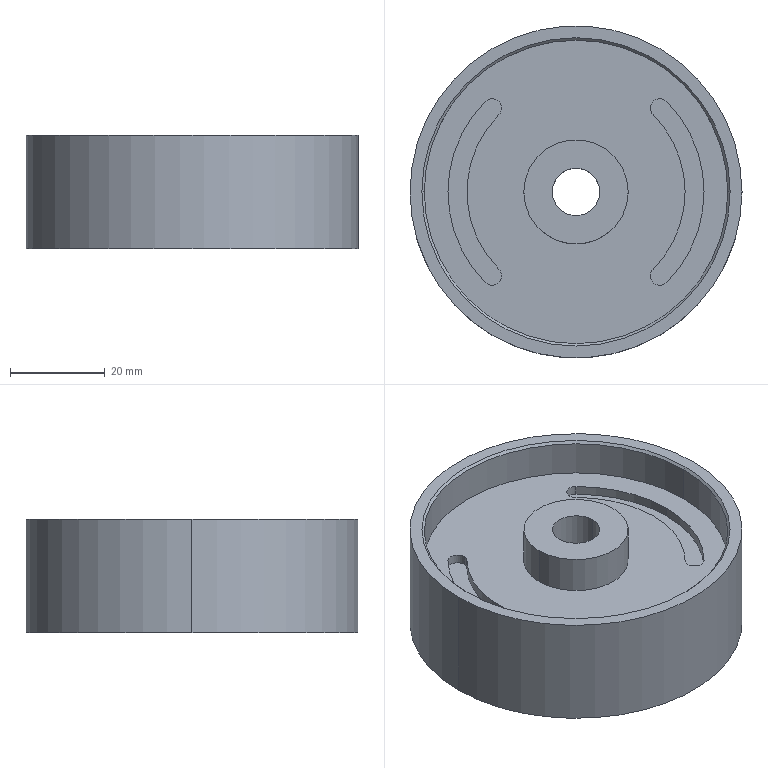Part | SolidWorks | features ICE 3, MirrorPattern 2, Chamfer 1, Extrusion 1 | 1 solid | 50 faces | box 70 x 70 x 24 mm | volume 43680 mm3 | cylinder 36 | plane 10 | cone 4 | commonest cylinder face diameters 4 x12 46 x6 54 x6 22 x4 64 x4 10 x2
STEP:
#1=CARTESIAN_POINT('',(-32.,0.,11.5));
#2=VERTEX_POINT('',#1);
#3=CARTESIAN_POINT('',(32.,0.,11.5));
#4=VERTEX_POINT('',#3);
#5=CARTESIAN_POINT('',(0.,0.,11.5));
#6=DIRECTION('',(0.,0.,1.));
#7=DIRECTION('',(1.,0.,0.));
#8=AXIS2_PLACEMENT_3D('',#5,#6,#7);
#9=CIRCLE('',#8,32.);
#10=EDGE_CURVE('',#2,#4,#9,.T.);
#11=ORIENTED_EDGE('',*,*,#10,.F.);
#12=CARTESIAN_POINT('',(-32.5,0.,12.));
#13=VERTEX_POINT('',#12);
#14=CARTESIAN_POINT('',(-32.,0.,11.5));
#15=DIRECTION('',(-0.7071,0.,0.7071));
#16=VECTOR('',#15,1000.);
#17=LINE('',#14,#16);
#18=EDGE_CURVE('',#2,#13,#17,.T.);
#19=ORIENTED_EDGE('',*,*,#18,.T.);
#20=CARTESIAN_POINT('',(32.5,0.,12.));
#21=VERTEX_POINT('',#20);
#22=CARTESIAN_POINT('',(0.,0.,12.));
#23=DIRECTION('',(0.,0.,-1.));
#24=DIRECTION('',(1.,0.,0.));
#25=AXIS2_PLACEMENT_3D('',#22,#23,#24);
#26=CIRCLE('',#25,32.5);
#27=EDGE_CURVE('',#21,#13,#26,.T.);
#28=ORIENTED_EDGE('',*,*,#27,.F.);
#29=CARTESIAN_POINT('',(32.,0.,11.5));
#30=DIRECTION('',(0.7071,0.,0.7071));
#31=VECTOR('',#30,1000.);
#32=LINE('',#29,#31);
#33=EDGE_CURVE('',#4,#21,#32,.T.);
#34=ORIENTED_EDGE('',*,*,#33,.F.);
#35=EDGE_LOOP('',(#11,#19,#28,#34));
#36=FACE_OUTER_BOUND('',#35,.T.);
#37=CARTESIAN_POINT('',(0.,0.,11.5));
#38=DIRECTION('',(0.,0.,1.));
#39=DIRECTION('',(1.,0.,0.));
#40=AXIS2_PLACEMENT_3D('',#37,#38,#39);
#41=CONICAL_SURFACE('',#40,32.,0.7854);
#42=ADVANCED_FACE('',(#36),#41,.F.);
#43=CARTESIAN_POINT('',(32.,0.,-11.5));
#44=VERTEX_POINT('',#43);
#45=CARTESIAN_POINT('',(-32.,0.,-11.5));
#46=VERTEX_POINT('',#45);
#47=CARTESIAN_POINT('',(0.,0.,-11.5));
#48=DIRECTION('',(0.,0.,-1.));
#49=DIRECTION('',(1.,0.,0.));
#50=AXIS2_PLACEMENT_3D('',#47,#48,#49);
#51=CIRCLE('',#50,32.);
#52=EDGE_CURVE('',#44,#46,#51,.T.);
#53=ORIENTED_EDGE('',*,*,#52,.F.);
#54=CARTESIAN_POINT('',(32.5,0.,-12.));
#55=VERTEX_POINT('',#54);
#56=CARTESIAN_POINT('',(32.5,0.,-12.));
#57=DIRECTION('',(0.7071,0.,-0.7071));
#58=VECTOR('',#57,1000.);
#59=LINE('',#56,#58);
#60=EDGE_CURVE('',#44,#55,#59,.T.);
#61=ORIENTED_EDGE('',*,*,#60,.T.);
#62=CARTESIAN_POINT('',(-32.5,0.,-12.));
#63=VERTEX_POINT('',#62);
#64=CARTESIAN_POINT('',(0.,0.,-12.));
#65=DIRECTION('',(0.,0.,1.));
#66=DIRECTION('',(1.,0.,0.));
#67=AXIS2_PLACEMENT_3D('',#64,#65,#66);
#68=CIRCLE('',#67,32.5);
#69=EDGE_CURVE('',#63,#55,#68,.T.);
#70=ORIENTED_EDGE('',*,*,#69,.F.);
#71=CARTESIAN_POINT('',(-32.5,0.,-12.));
#72=DIRECTION('',(-0.7071,0.,-0.7071));
#73=VECTOR('',#72,1000.);
#74=LINE('',#71,#73);
#75=EDGE_CURVE('',#46,#63,#74,.T.);
#76=ORIENTED_EDGE('',*,*,#75,.F.);
#77=EDGE_LOOP('',(#53,#61,#70,#76));
#78=FACE_OUTER_BOUND('',#77,.T.);
#79=CARTESIAN_POINT('',(0.,0.,-12.));
#80=DIRECTION('',(0.,0.,-1.));
#81=DIRECTION('',(-1.,0.,0.));
#82=AXIS2_PLACEMENT_3D('',#79,#80,#81);
#83=CONICAL_SURFACE('',#82,32.5,0.7854);
#84=ADVANCED_FACE('',(#78),#83,.F.);
#85=CARTESIAN_POINT('',(-19.092,19.092,2.));
#86=VERTEX_POINT('',#85);
#87=CARTESIAN_POINT('',(-15.678,17.678,2.));
#88=VERTEX_POINT('',#87);
#89=CARTESIAN_POINT('',(-17.678,17.678,2.));
#90=DIRECTION('',(0.,0.,-1.));
#91=DIRECTION('',(-1.,0.,0.));
#92=AXIS2_PLACEMENT_3D('',#89,#90,#91);
#93=CIRCLE('',#92,2.);
#94=EDGE_CURVE('',#86,#88,#93,.T.);
#95=ORIENTED_EDGE('',*,*,#94,.T.);
#96=CARTESIAN_POINT('',(-15.678,17.678,4.));
#97=VERTEX_POINT('',#96);
#98=CARTESIAN_POINT('',(-15.678,17.678,2.));
#99=DIRECTION('',(0.,0.,1.));
#100=VECTOR('',#99,1000.);
#101=LINE('',#98,#100);
#102=EDGE_CURVE('',#88,#97,#101,.T.);
#103=ORIENTED_EDGE('',*,*,#102,.T.);
#104=CARTESIAN_POINT('',(-19.092,19.092,4.));
#105=VERTEX_POINT('',#104);
#106=CARTESIAN_POINT('',(-17.678,17.678,4.));
#107=DIRECTION('',(0.,0.,-1.));
#108=DIRECTION('',(-1.,0.,0.));
#109=AXIS2_PLACEMENT_3D('',#106,#107,#108);
#110=CIRCLE('',#109,2.);
#111=EDGE_CURVE('',#105,#97,#110,.T.);
#112=ORIENTED_EDGE('',*,*,#111,.F.);
#113=CARTESIAN_POINT('',(-19.092,19.092,2.));
#114=DIRECTION('',(0.,0.,1.));
#115=VECTOR('',#114,1000.);
#116=LINE('',#113,#115);
#117=EDGE_CURVE('',#86,#105,#116,.T.);
#118=ORIENTED_EDGE('',*,*,#117,.F.);
#119=EDGE_LOOP('',(#95,#103,#112,#118));
#120=FACE_OUTER_BOUND('',#119,.T.);
#121=CARTESIAN_POINT('',(-17.678,17.678,2.));
#122=DIRECTION('',(0.,0.,1.));
#123=DIRECTION('',(1.,0.,0.));
#124=AXIS2_PLACEMENT_3D('',#121,#122,#123);
#125=CYLINDRICAL_SURFACE('',#124,2.);
#126=ADVANCED_FACE('',(#120),#125,.F.);
#127=CARTESIAN_POINT('',(-16.263,-16.263,2.));
#128=VERTEX_POINT('',#127);
#129=CARTESIAN_POINT('',(-15.678,-17.678,2.));
#130=VERTEX_POINT('',#129);
#131=CARTESIAN_POINT('',(-17.678,-17.678,2.));
#132=DIRECTION('',(0.,0.,-1.));
#133=DIRECTION('',(-1.,0.,0.));
#134=AXIS2_PLACEMENT_3D('',#131,#132,#133);
#135=CIRCLE('',#134,2.);
#136=EDGE_CURVE('',#128,#130,#135,.T.);
#137=ORIENTED_EDGE('',*,*,#136,.T.);
#138=CARTESIAN_POINT('',(-15.678,-17.678,4.));
#139=VERTEX_POINT('',#138);
#140=CARTESIAN_POINT('',(-15.678,-17.678,2.));
#141=DIRECTION('',(0.,0.,1.));
#142=VECTOR('',#141,1000.);
#143=LINE('',#140,#142);
#144=EDGE_CURVE('',#130,#139,#143,.T.);
#145=ORIENTED_EDGE('',*,*,#144,.T.);
#146=CARTESIAN_POINT('',(-16.263,-16.263,4.));
#147=VERTEX_POINT('',#146);
#148=CARTESIAN_POINT('',(-17.678,-17.678,4.));
#149=DIRECTION('',(0.,0.,-1.));
#150=DIRECTION('',(-1.,0.,0.));
#151=AXIS2_PLACEMENT_3D('',#148,#149,#150);
#152=CIRCLE('',#151,2.);
#153=EDGE_CURVE('',#147,#139,#152,.T.);
#154=ORIENTED_EDGE('',*,*,#153,.F.);
#155=CARTESIAN_POINT('',(-16.263,-16.263,2.));
#156=DIRECTION('',(0.,0.,1.));
#157=VECTOR('',#156,1000.);
#158=LINE('',#155,#157);
#159=EDGE_CURVE('',#128,#147,#158,.T.);
#160=ORIENTED_EDGE('',*,*,#159,.F.);
#161=EDGE_LOOP('',(#137,#145,#154,#160));
#162=FACE_OUTER_BOUND('',#161,.T.);
#163=CARTESIAN_POINT('',(-17.678,-17.678,2.));
#164=DIRECTION('',(0.,0.,1.));
#165=DIRECTION('',(1.,0.,0.));
#166=AXIS2_PLACEMENT_3D('',#163,#164,#165);
#167=CYLINDRICAL_SURFACE('',#166,2.);
#168=ADVANCED_FACE('',(#162),#167,.F.);
#169=CARTESIAN_POINT('',(19.092,19.092,2.));
#170=VERTEX_POINT('',#169);
#171=CARTESIAN_POINT('',(27.,0.,2.));
#172=VERTEX_POINT('',#171);
#173=CARTESIAN_POINT('',(0.,0.,2.));
#174=DIRECTION('',(0.,0.,-1.));
#175=DIRECTION('',(1.,0.,0.));
#176=AXIS2_PLACEMENT_3D('',#173,#174,#175);
#177=CIRCLE('',#176,27.);
#178=EDGE_CURVE('',#170,#172,#177,.T.);
#179=ORIENTED_EDGE('',*,*,#178,.T.);
#180=CARTESIAN_POINT('',(27.,0.,4.));
#181=VERTEX_POINT('',#180);
#182=CARTESIAN_POINT('',(27.,0.,2.));
#183=DIRECTION('',(0.,0.,1.));
#184=VECTOR('',#183,1000.);
#185=LINE('',#182,#184);
#186=EDGE_CURVE('',#172,#181,#185,.T.);
#187=ORIENTED_EDGE('',*,*,#186,.T.);
#188=CARTESIAN_POINT('',(19.092,19.092,4.));
#189=VERTEX_POINT('',#188);
#190=CARTESIAN_POINT('',(0.,0.,4.));
#191=DIRECTION('',(0.,0.,-1.));
#192=DIRECTION('',(1.,0.,0.));
#193=AXIS2_PLACEMENT_3D('',#190,#191,#192);
#194=CIRCLE('',#193,27.);
#195=EDGE_CURVE('',#189,#181,#194,.T.);
#196=ORIENTED_EDGE('',*,*,#195,.F.);
#197=CARTESIAN_POINT('',(19.092,19.092,2.));
#198=DIRECTION('',(0.,0.,1.));
#199=VECTOR('',#198,1000.);
#200=LINE('',#197,#199);
#201=EDGE_CURVE('',#170,#189,#200,.T.);
#202=ORIENTED_EDGE('',*,*,#201,.F.);
#203=EDGE_LOOP('',(#179,#187,#196,#202));
#204=FACE_OUTER_BOUND('',#203,.T.);
#205=CARTESIAN_POINT('',(0.,0.,2.));
#206=DIRECTION('',(0.,0.,1.));
#207=DIRECTION('',(1.,0.,0.));
#208=AXIS2_PLACEMENT_3D('',#205,#206,#207);
#209=CYLINDRICAL_SURFACE('',#208,27.);
#210=ADVANCED_FACE('',(#204),#209,.F.);
#211=CARTESIAN_POINT('',(16.263,-16.263,2.));
#212=VERTEX_POINT('',#211);
#213=CARTESIAN_POINT('',(23.,0.,2.));
#214=VERTEX_POINT('',#213);
#215=CARTESIAN_POINT('',(0.,0.,2.));
#216=DIRECTION('',(0.,0.,1.));
#217=DIRECTION('',(1.,0.,0.));
#218=AXIS2_PLACEMENT_3D('',#215,#216,#217);
#219=CIRCLE('',#218,23.);
#220=EDGE_CURVE('',#212,#214,#219,.T.);
#221=ORIENTED_EDGE('',*,*,#220,.T.);
#222=CARTESIAN_POINT('',(23.,0.,4.));
#223=VERTEX_POINT('',#222);
#224=CARTESIAN_POINT('',(23.,0.,2.));
#225=DIRECTION('',(0.,0.,1.));
#226=VECTOR('',#225,1000.);
#227=LINE('',#224,#226);
#228=EDGE_CURVE('',#214,#223,#227,.T.);
#229=ORIENTED_EDGE('',*,*,#228,.T.);
#230=CARTESIAN_POINT('',(16.263,-16.263,4.));
#231=VERTEX_POINT('',#230);
#232=CARTESIAN_POINT('',(0.,0.,4.));
#233=DIRECTION('',(0.,0.,1.));
#234=DIRECTION('',(1.,0.,0.));
#235=AXIS2_PLACEMENT_3D('',#232,#233,#234);
#236=CIRCLE('',#235,23.);
#237=EDGE_CURVE('',#231,#223,#236,.T.);
#238=ORIENTED_EDGE('',*,*,#237,.F.);
#239=CARTESIAN_POINT('',(16.263,-16.263,2.));
#240=DIRECTION('',(0.,0.,1.));
#241=VECTOR('',#240,1000.);
#242=LINE('',#239,#241);
#243=EDGE_CURVE('',#212,#231,#242,.T.);
#244=ORIENTED_EDGE('',*,*,#243,.F.);
#245=EDGE_LOOP('',(#221,#229,#238,#244));
#246=FACE_OUTER_BOUND('',#245,.T.);
#247=CARTESIAN_POINT('',(0.,0.,2.));
#248=DIRECTION('',(0.,0.,1.));
#249=DIRECTION('',(1.,0.,0.));
#250=AXIS2_PLACEMENT_3D('',#247,#248,#249);
#251=CYLINDRICAL_SURFACE('',#250,23.);
#252=ADVANCED_FACE('',(#246),#251,.T.);
#253=CARTESIAN_POINT('',(-27.,0.,-2.));
#254=VERTEX_POINT('',#253);
#255=CARTESIAN_POINT('',(-19.092,19.092,-2.));
#256=VERTEX_POINT('',#255);
#257=CARTESIAN_POINT('',(0.,0.,-2.));
#258=DIRECTION('',(0.,0.,-1.));
#259=DIRECTION('',(-1.,0.,0.));
#260=AXIS2_PLACEMENT_3D('',#257,#258,#259);
#261=CIRCLE('',#260,27.);
#262=EDGE_CURVE('',#254,#256,#261,.T.);
#263=ORIENTED_EDGE('',*,*,#262,.F.);
#264=CARTESIAN_POINT('',(-27.,0.,-4.));
#265=VERTEX_POINT('',#264);
#266=CARTESIAN_POINT('',(-27.,0.,-2.));
#267=DIRECTION('',(0.,0.,-1.));
#268=VECTOR('',#267,1000.);
#269=LINE('',#266,#268);
#270=EDGE_CURVE('',#254,#265,#269,.T.);
#271=ORIENTED_EDGE('',*,*,#270,.T.);
#272=CARTESIAN_POINT('',(-19.092,19.092,-4.));
#273=VERTEX_POINT('',#272);
#274=CARTESIAN_POINT('',(0.,0.,-4.));
#275=DIRECTION('',(0.,0.,-1.));
#276=DIRECTION('',(-1.,0.,0.));
#277=AXIS2_PLACEMENT_3D('',#274,#275,#276);
#278=CIRCLE('',#277,27.);
#279=EDGE_CURVE('',#265,#273,#278,.T.);
#280=ORIENTED_EDGE('',*,*,#279,.T.);
#281=CARTESIAN_POINT('',(-19.092,19.092,-2.));
#282=DIRECTION('',(0.,0.,-1.));
#283=VECTOR('',#282,1000.);
#284=LINE('',#281,#283);
#285=EDGE_CURVE('',#256,#273,#284,.T.);
#286=ORIENTED_EDGE('',*,*,#285,.F.);
#287=EDGE_LOOP('',(#263,#271,#280,#286));
#288=FACE_OUTER_BOUND('',#287,.T.);
#289=CARTESIAN_POINT('',(0.,0.,-2.));
#290=DIRECTION('',(0.,0.,-1.));
#291=DIRECTION('',(-1.,0.,0.));
#292=AXIS2_PLACEMENT_3D('',#289,#290,#291);
#293=CYLINDRICAL_SURFACE('',#292,27.);
#294=ADVANCED_FACE('',(#288),#293,.F.);
#295=CARTESIAN_POINT('',(-23.,0.,-2.));
#296=VERTEX_POINT('',#295);
#297=CARTESIAN_POINT('',(-16.263,-16.263,-2.));
#298=VERTEX_POINT('',#297);
#299=CARTESIAN_POINT('',(0.,0.,-2.));
#300=DIRECTION('',(0.,0.,1.));
#301=DIRECTION('',(-1.,0.,0.));
#302=AXIS2_PLACEMENT_3D('',#299,#300,#301);
#303=CIRCLE('',#302,23.);
#304=EDGE_CURVE('',#296,#298,#303,.T.);
#305=ORIENTED_EDGE('',*,*,#304,.F.);
#306=CARTESIAN_POINT('',(-23.,0.,-4.));
#307=VERTEX_POINT('',#306);
#308=CARTESIAN_POINT('',(-23.,0.,-2.));
#309=DIRECTION('',(0.,0.,-1.));
#310=VECTOR('',#309,1000.);
#311=LINE('',#308,#310);
#312=EDGE_CURVE('',#296,#307,#311,.T.);
#313=ORIENTED_EDGE('',*,*,#312,.T.);
#314=CARTESIAN_POINT('',(-16.263,-16.263,-4.));
#315=VERTEX_POINT('',#314);
#316=CARTESIAN_POINT('',(0.,0.,-4.));
#317=DIRECTION('',(0.,0.,1.));
#318=DIRECTION('',(-1.,0.,0.));
#319=AXIS2_PLACEMENT_3D('',#316,#317,#318);
#320=CIRCLE('',#319,23.);
#321=EDGE_CURVE('',#307,#315,#320,.T.);
#322=ORIENTED_EDGE('',*,*,#321,.T.);
#323=CARTESIAN_POINT('',(-16.263,-16.263,-2.));
#324=DIRECTION('',(0.,0.,-1.));
#325=VECTOR('',#324,1000.);
#326=LINE('',#323,#325);
#327=EDGE_CURVE('',#298,#315,#326,.T.);
#328=ORIENTED_EDGE('',*,*,#327,.F.);
#329=EDGE_LOOP('',(#305,#313,#322,#328));
#330=FACE_OUTER_BOUND('',#329,.T.);
#331=CARTESIAN_POINT('',(0.,0.,-2.));
#332=DIRECTION('',(0.,0.,-1.));
#333=DIRECTION('',(-1.,0.,0.));
#334=AXIS2_PLACEMENT_3D('',#331,#332,#333);
#335=CYLINDRICAL_SURFACE('',#334,23.);
#336=ADVANCED_FACE('',(#330),#335,.T.);
#337=CARTESIAN_POINT('',(15.678,17.678,-2.));
#338=VERTEX_POINT('',#337);
#339=CARTESIAN_POINT('',(19.092,19.092,-2.));
#340=VERTEX_POINT('',#339);
#341=CARTESIAN_POINT('',(17.678,17.678,-2.));
#342=DIRECTION('',(0.,0.,-1.));
#343=DIRECTION('',(1.,0.,0.));
#344=AXIS2_PLACEMENT_3D('',#341,#342,#343);
#345=CIRCLE('',#344,2.);
#346=EDGE_CURVE('',#338,#340,#345,.T.);
#347=ORIENTED_EDGE('',*,*,#346,.F.);
#348=CARTESIAN_POINT('',(15.678,17.678,-4.));
#349=VERTEX_POINT('',#348);
#350=CARTESIAN_POINT('',(15.678,17.678,-2.));
#351=DIRECTION('',(0.,0.,-1.));
#352=VECTOR('',#351,1000.);
#353=LINE('',#350,#352);
#354=EDGE_CURVE('',#338,#349,#353,.T.);
#355=ORIENTED_EDGE('',*,*,#354,.T.);
#356=CARTESIAN_POINT('',(19.092,19.092,-4.));
#357=VERTEX_POINT('',#356);
#358=CARTESIAN_POINT('',(17.678,17.678,-4.));
#359=DIRECTION('',(0.,0.,-1.));
#360=DIRECTION('',(1.,0.,0.));
#361=AXIS2_PLACEMENT_3D('',#358,#359,#360);
#362=CIRCLE('',#361,2.);
#363=EDGE_CURVE('',#349,#357,#362,.T.);
#364=ORIENTED_EDGE('',*,*,#363,.T.);
#365=CARTESIAN_POINT('',(19.092,19.092,-2.));
#366=DIRECTION('',(0.,0.,-1.));
#367=VECTOR('',#366,1000.);
#368=LINE('',#365,#367);
#369=EDGE_CURVE('',#340,#357,#368,.T.);
#370=ORIENTED_EDGE('',*,*,#369,.F.);
#371=EDGE_LOOP('',(#347,#355,#364,#370));
#372=FACE_OUTER_BOUND('',#371,.T.);
#373=CARTESIAN_POINT('',(17.678,17.678,-2.));
#374=DIRECTION('',(0.,0.,-1.));
#375=DIRECTION('',(-1.,0.,0.));
#376=AXIS2_PLACEMENT_3D('',#373,#374,#375);
#377=CYLINDRICAL_SURFACE('',#376,2.);
#378=ADVANCED_FACE('',(#372),#377,.F.);
#379=CARTESIAN_POINT('',(15.678,-17.678,-2.));
#380=VERTEX_POINT('',#379);
#381=CARTESIAN_POINT('',(16.263,-16.263,-2.));
#382=VERTEX_POINT('',#381);
#383=CARTESIAN_POINT('',(17.678,-17.678,-2.));
#384=DIRECTION('',(0.,0.,-1.));
#385=DIRECTION('',(1.,0.,0.));
#386=AXIS2_PLACEMENT_3D('',#383,#384,#385);
#387=CIRCLE('',#386,2.);
#388=EDGE_CURVE('',#380,#382,#387,.T.);
#389=ORIENTED_EDGE('',*,*,#388,.F.);
#390=CARTESIAN_POINT('',(15.678,-17.678,-4.));
#391=VERTEX_POINT('',#390);
#392=CARTESIAN_POINT('',(15.678,-17.678,-2.));
#393=DIRECTION('',(0.,0.,-1.));
#394=VECTOR('',#393,1000.);
#395=LINE('',#392,#394);
#396=EDGE_CURVE('',#380,#391,#395,.T.);
#397=ORIENTED_EDGE('',*,*,#396,.T.);
#398=CARTESIAN_POINT('',(16.263,-16.263,-4.));
#399=VERTEX_POINT('',#398);
#400=CARTESIAN_POINT('',(17.678,-17.678,-4.));
#401=DIRECTION('',(0.,0.,-1.));
#402=DIRECTION('',(1.,0.,0.));
#403=AXIS2_PLACEMENT_3D('',#400,#401,#402);
#404=CIRCLE('',#403,2.);
#405=EDGE_CURVE('',#391,#399,#404,.T.);
#406=ORIENTED_EDGE('',*,*,#405,.T.);
#407=CARTESIAN_POINT('',(16.263,-16.263,-2.));
#408=DIRECTION('',(0.,0.,-1.));
#409=VECTOR('',#408,1000.);
#410=LINE('',#407,#409);
#411=EDGE_CURVE('',#382,#399,#410,.T.);
#412=ORIENTED_EDGE('',*,*,#411,.F.);
#413=EDGE_LOOP('',(#389,#397,#406,#412));
#414=FACE_OUTER_BOUND('',#413,.T.);
#415=CARTESIAN_POINT('',(17.678,-17.678,-2.));
#416=DIRECTION('',(0.,0.,-1.));
#417=DIRECTION('',(-1.,0.,0.));
#418=AXIS2_PLACEMENT_3D('',#415,#416,#417);
#419=CYLINDRICAL_SURFACE('',#418,2.);
#420=ADVANCED_FACE('',(#414),#419,.F.);
#421=CARTESIAN_POINT('',(11.,0.,-4.));
#422=VERTEX_POINT('',#421);
#423=CARTESIAN_POINT('',(-11.,0.,-4.));
#424=VERTEX_POINT('',#423);
#425=CARTESIAN_POINT('',(0.,0.,-4.));
#426=DIRECTION('',(0.,0.,1.));
#427=DIRECTION('',(1.,0.,0.));
#428=AXIS2_PLACEMENT_3D('',#425,#426,#427);
#429=CIRCLE('',#428,11.);
#430=EDGE_CURVE('',#422,#424,#429,.T.);
#431=ORIENTED_EDGE('',*,*,#430,.F.);
#432=CARTESIAN_POINT('',(11.,0.,-12.));
#433=VERTEX_POINT('',#432);
#434=CARTESIAN_POINT('',(11.,0.,-4.));
#435=DIRECTION('',(0.,0.,-1.));
#436=VECTOR('',#435,1000.);
#437=LINE('',#434,#436);
#438=EDGE_CURVE('',#422,#433,#437,.T.);
#439=ORIENTED_EDGE('',*,*,#438,.T.);
#440=CARTESIAN_POINT('',(-11.,0.,-12.));
#441=VERTEX_POINT('',#440);
#442=CARTESIAN_POINT('',(0.,0.,-12.));
#443=DIRECTION('',(0.,0.,1.));
#444=DIRECTION('',(1.,0.,0.));
#445=AXIS2_PLACEMENT_3D('',#442,#443,#444);
#446=CIRCLE('',#445,11.);
#447=EDGE_CURVE('',#433,#441,#446,.T.);
#448=ORIENTED_EDGE('',*,*,#447,.T.);
#449=CARTESIAN_POINT('',(-11.,0.,-4.));
#450=DIRECTION('',(0.,0.,-1.));
#451=VECTOR('',#450,1000.);
#452=LINE('',#449,#451);
#453=EDGE_CURVE('',#424,#441,#452,.T.);
#454=ORIENTED_EDGE('',*,*,#453,.F.);
#455=EDGE_LOOP('',(#431,#439,#448,#454));
#456=FACE_OUTER_BOUND('',#455,.T.);
#457=CARTESIAN_POINT('',(0.,0.,-4.));
#458=DIRECTION('',(0.,0.,-1.));
#459=DIRECTION('',(-1.,0.,0.));
#460=AXIS2_PLACEMENT_3D('',#457,#458,#459);
#461=CYLINDRICAL_SURFACE('',#460,11.);
#462=ADVANCED_FACE('',(#456),#461,.T.);
#463=CARTESIAN_POINT('',(-32.,0.,-4.));
#464=VERTEX_POINT('',#463);
#465=CARTESIAN_POINT('',(32.,0.,-4.));
#466=VERTEX_POINT('',#465);
#467=CARTESIAN_POINT('',(0.,0.,-4.));
#468=DIRECTION('',(0.,0.,1.));
#469=DIRECTION('',(1.,0.,0.));
#470=AXIS2_PLACEMENT_3D('',#467,#468,#469);
#471=CIRCLE('',#470,32.);
#472=EDGE_CURVE('',#464,#466,#471,.T.);
#473=ORIENTED_EDGE('',*,*,#472,.T.);
#474=CARTESIAN_POINT('',(32.,0.,-4.));
#475=DIRECTION('',(0.,0.,-1.));
#476=VECTOR('',#475,1000.);
#477=LINE('',#474,#476);
#478=EDGE_CURVE('',#466,#44,#477,.T.);
#479=ORIENTED_EDGE('',*,*,#478,.T.);
#480=ORIENTED_EDGE('',*,*,#52,.T.);
#481=CARTESIAN_POINT('',(-32.,0.,-4.));
#482=DIRECTION('',(0.,0.,-1.));
#483=VECTOR('',#482,1000.);
#484=LINE('',#481,#483);
#485=EDGE_CURVE('',#464,#46,#484,.T.);
#486=ORIENTED_EDGE('',*,*,#485,.F.);
#487=EDGE_LOOP('',(#473,#479,#480,#486));
#488=FACE_OUTER_BOUND('',#487,.T.);
#489=CARTESIAN_POINT('',(0.,0.,-4.));
#490=DIRECTION('',(0.,0.,-1.));
#491=DIRECTION('',(-1.,0.,0.));
#492=AXIS2_PLACEMENT_3D('',#489,#490,#491);
#493=CYLINDRICAL_SURFACE('',#492,32.);
#494=ADVANCED_FACE('',(#488),#493,.F.);
#495=CARTESIAN_POINT('',(11.,0.,4.));
#496=VERTEX_POINT('',#495);
#497=CARTESIAN_POINT('',(-11.,0.,4.));
#498=VERTEX_POINT('',#497);
#499=CARTESIAN_POINT('',(0.,0.,4.));
#500=DIRECTION('',(0.,0.,1.));
#501=DIRECTION('',(1.,0.,0.));
#502=AXIS2_PLACEMENT_3D('',#499,#500,#501);
#503=CIRCLE('',#502,11.);
#504=EDGE_CURVE('',#496,#498,#503,.T.);
#505=ORIENTED_EDGE('',*,*,#504,.T.);
#506=CARTESIAN_POINT('',(-11.,0.,12.));
#507=VERTEX_POINT('',#506);
#508=CARTESIAN_POINT('',(-11.,0.,4.));
#509=DIRECTION('',(0.,0.,1.));
#510=VECTOR('',#509,1000.);
#511=LINE('',#508,#510);
#512=EDGE_CURVE('',#498,#507,#511,.T.);
#513=ORIENTED_EDGE('',*,*,#512,.T.);
#514=CARTESIAN_POINT('',(11.,0.,12.));
#515=VERTEX_POINT('',#514);
#516=CARTESIAN_POINT('',(0.,0.,12.));
#517=DIRECTION('',(0.,0.,1.));
#518=DIRECTION('',(1.,0.,0.));
#519=AXIS2_PLACEMENT_3D('',#516,#517,#518);
#520=CIRCLE('',#519,11.);
#521=EDGE_CURVE('',#515,#507,#520,.T.);
#522=ORIENTED_EDGE('',*,*,#521,.F.);
#523=CARTESIAN_POINT('',(11.,0.,4.));
#524=DIRECTION('',(0.,0.,1.));
#525=VECTOR('',#524,1000.);
#526=LINE('',#523,#525);
#527=EDGE_CURVE('',#496,#515,#526,.T.);
#528=ORIENTED_EDGE('',*,*,#527,.F.);
#529=EDGE_LOOP('',(#505,#513,#522,#528));
#530=FACE_OUTER_BOUND('',#529,.T.);
#531=CARTESIAN_POINT('',(0.,0.,4.));
#532=DIRECTION('',(0.,0.,1.));
#533=DIRECTION('',(1.,0.,0.));
#534=AXIS2_PLACEMENT_3D('',#531,#532,#533);
#535=CYLINDRICAL_SURFACE('',#534,11.);
#536=ADVANCED_FACE('',(#530),#535,.T.);
#537=CARTESIAN_POINT('',(-32.,0.,4.));
#538=VERTEX_POINT('',#537);
#539=CARTESIAN_POINT('',(32.,0.,4.));
#540=VERTEX_POINT('',#539);
#541=CARTESIAN_POINT('',(0.,0.,4.));
#542=DIRECTION('',(0.,0.,1.));
#543=DIRECTION('',(1.,0.,0.));
#544=AXIS2_PLACEMENT_3D('',#541,#542,#543);
#545=CIRCLE('',#544,32.);
#546=EDGE_CURVE('',#538,#540,#545,.T.);
#547=ORIENTED_EDGE('',*,*,#546,.F.);
#548=CARTESIAN_POINT('',(-32.,0.,4.));
#549=DIRECTION('',(0.,0.,1.));
#550=VECTOR('',#549,1000.);
#551=LINE('',#548,#550);
#552=EDGE_CURVE('',#538,#2,#551,.T.);
#553=ORIENTED_EDGE('',*,*,#552,.T.);
#554=ORIENTED_EDGE('',*,*,#10,.T.);
#555=CARTESIAN_POINT('',(32.,0.,4.));
#556=DIRECTION('',(0.,0.,1.));
#557=VECTOR('',#556,1000.);
#558=LINE('',#555,#557);
#559=EDGE_CURVE('',#540,#4,#558,.T.);
#560=ORIENTED_EDGE('',*,*,#559,.F.);
#561=EDGE_LOOP('',(#547,#553,#554,#560));
#562=FACE_OUTER_BOUND('',#561,.T.);
#563=CARTESIAN_POINT('',(0.,0.,4.));
#564=DIRECTION('',(0.,0.,1.));
#565=DIRECTION('',(1.,0.,0.));
#566=AXIS2_PLACEMENT_3D('',#563,#564,#565);
#567=CYLINDRICAL_SURFACE('',#566,32.);
#568=ADVANCED_FACE('',(#562),#567,.F.);
#569=CARTESIAN_POINT('',(-5.,0.,-12.));
#570=VERTEX_POINT('',#569);
#571=CARTESIAN_POINT('',(5.,0.,-12.));
#572=VERTEX_POINT('',#571);
#573=CARTESIAN_POINT('',(0.,0.,-12.));
#574=DIRECTION('',(0.,0.,1.));
#575=DIRECTION('',(1.,0.,0.));
#576=AXIS2_PLACEMENT_3D('',#573,#574,#575);
#577=CIRCLE('',#576,5.);
#578=EDGE_CURVE('',#570,#572,#577,.T.);
#579=ORIENTED_EDGE('',*,*,#578,.F.);
#580=CARTESIAN_POINT('',(-5.,0.,12.));
#581=VERTEX_POINT('',#580);
#582=CARTESIAN_POINT('',(-5.,0.,-58.5));
#583=DIRECTION('',(0.,0.,1.));
#584=VECTOR('',#583,1000.);
#585=LINE('',#582,#584);
#586=EDGE_CURVE('',#570,#581,#585,.T.);
#587=ORIENTED_EDGE('',*,*,#586,.T.);
#588=CARTESIAN_POINT('',(5.,0.,12.));
#589=VERTEX_POINT('',#588);
#590=CARTESIAN_POINT('',(0.,0.,12.));
#591=DIRECTION('',(0.,0.,1.));
#592=DIRECTION('',(1.,0.,0.));
#593=AXIS2_PLACEMENT_3D('',#590,#591,#592);
#594=CIRCLE('',#593,5.);
#595=EDGE_CURVE('',#581,#589,#594,.T.);
#596=ORIENTED_EDGE('',*,*,#595,.T.);
#597=CARTESIAN_POINT('',(5.,0.,-58.5));
#598=DIRECTION('',(0.,0.,1.));
#599=VECTOR('',#598,1000.);
#600=LINE('',#597,#599);
#601=EDGE_CURVE('',#572,#589,#600,.T.);
#602=ORIENTED_EDGE('',*,*,#601,.F.);
#603=EDGE_LOOP('',(#579,#587,#596,#602));
#604=FACE_OUTER_BOUND('',#603,.T.);
#605=CARTESIAN_POINT('',(0.,0.,-58.5));
#606=DIRECTION('',(0.,0.,1.));
#607=DIRECTION('',(1.,0.,0.));
#608=AXIS2_PLACEMENT_3D('',#605,#606,#607);
#609=CYLINDRICAL_SURFACE('',#608,5.);
#610=ADVANCED_FACE('',(#604),#609,.F.);
#611=CARTESIAN_POINT('',(35.,0.,12.));
#612=VERTEX_POINT('',#611);
#613=CARTESIAN_POINT('',(-35.,0.,12.));
#614=VERTEX_POINT('',#613);
#615=CARTESIAN_POINT('',(0.,0.,12.));
#616=DIRECTION('',(0.,0.,1.));
#617=DIRECTION('',(1.,0.,0.));
#618=AXIS2_PLACEMENT_3D('',#615,#616,#617);
#619=CIRCLE('',#618,35.);
#620=EDGE_CURVE('',#612,#614,#619,.T.);
#621=ORIENTED_EDGE('',*,*,#620,.F.);
#622=CARTESIAN_POINT('',(35.,0.,-12.));
#623=VERTEX_POINT('',#622);
#624=CARTESIAN_POINT('',(35.,0.,12.));
#625=DIRECTION('',(0.,0.,-1.));
#626=VECTOR('',#625,1000.);
#627=LINE('',#624,#626);
#628=EDGE_CURVE('',#612,#623,#627,.T.);
#629=ORIENTED_EDGE('',*,*,#628,.T.);
#630=CARTESIAN_POINT('',(-35.,0.,-12.));
#631=VERTEX_POINT('',#630);
#632=CARTESIAN_POINT('',(0.,0.,-12.));
#633=DIRECTION('',(0.,0.,1.));
#634=DIRECTION('',(1.,0.,0.));
#635=AXIS2_PLACEMENT_3D('',#632,#633,#634);
#636=CIRCLE('',#635,35.);
#637=EDGE_CURVE('',#623,#631,#636,.T.);
#638=ORIENTED_EDGE('',*,*,#637,.T.);
#639=CARTESIAN_POINT('',(-35.,0.,12.));
#640=DIRECTION('',(0.,0.,-1.));
#641=VECTOR('',#640,1000.);
#642=LINE('',#639,#641);
#643=EDGE_CURVE('',#614,#631,#642,.T.);
#644=ORIENTED_EDGE('',*,*,#643,.F.);
#645=EDGE_LOOP('',(#621,#629,#638,#644));
#646=FACE_OUTER_BOUND('',#645,.T.);
#647=CARTESIAN_POINT('',(0.,0.,12.));
#648=DIRECTION('',(0.,0.,-1.));
#649=DIRECTION('',(-1.,0.,0.));
#650=AXIS2_PLACEMENT_3D('',#647,#648,#649);
#651=CYLINDRICAL_SURFACE('',#650,35.);
#652=ADVANCED_FACE('',(#646),#651,.T.);
#653=CARTESIAN_POINT('',(19.092,-19.092,-4.));
#654=VERTEX_POINT('',#653);
#655=CARTESIAN_POINT('',(17.678,-17.678,-4.));
#656=DIRECTION('',(0.,0.,-1.));
#657=DIRECTION('',(1.,0.,0.));
#658=AXIS2_PLACEMENT_3D('',#655,#656,#657);
#659=CIRCLE('',#658,2.);
#660=EDGE_CURVE('',#654,#391,#659,.T.);
#661=ORIENTED_EDGE('',*,*,#660,.F.);
#662=CARTESIAN_POINT('',(0.,0.,-4.));
#663=DIRECTION('',(0.,0.,-1.));
#664=DIRECTION('',(1.,0.,0.));
#665=AXIS2_PLACEMENT_3D('',#662,#663,#664);
#666=CIRCLE('',#665,27.);
#667=EDGE_CURVE('',#357,#654,#666,.T.);
#668=ORIENTED_EDGE('',*,*,#667,.F.);
#669=ORIENTED_EDGE('',*,*,#363,.F.);
#670=CARTESIAN_POINT('',(16.263,16.263,-4.));
#671=VERTEX_POINT('',#670);
#672=CARTESIAN_POINT('',(17.678,17.678,-4.));
#673=DIRECTION('',(0.,0.,-1.));
#674=DIRECTION('',(1.,0.,0.));
#675=AXIS2_PLACEMENT_3D('',#672,#673,#674);
#676=CIRCLE('',#675,2.);
#677=EDGE_CURVE('',#671,#349,#676,.T.);
#678=ORIENTED_EDGE('',*,*,#677,.F.);
#679=CARTESIAN_POINT('',(0.,0.,-4.));
#680=DIRECTION('',(0.,0.,1.));
#681=DIRECTION('',(1.,0.,0.));
#682=AXIS2_PLACEMENT_3D('',#679,#680,#681);
#683=CIRCLE('',#682,23.);
#684=EDGE_CURVE('',#399,#671,#683,.T.);
#685=ORIENTED_EDGE('',*,*,#684,.F.);
#686=ORIENTED_EDGE('',*,*,#405,.F.);
#687=EDGE_LOOP('',(#661,#668,#669,#678,#685,#686));
#688=FACE_BOUND('',#687,.T.);
#689=ORIENTED_EDGE('',*,*,#472,.F.);
#690=CARTESIAN_POINT('',(0.,0.,-4.));
#691=DIRECTION('',(0.,0.,1.));
#692=DIRECTION('',(1.,0.,0.));
#693=AXIS2_PLACEMENT_3D('',#690,#691,#692);
#694=CIRCLE('',#693,32.);
#695=EDGE_CURVE('',#466,#464,#694,.T.);
#696=ORIENTED_EDGE('',*,*,#695,.F.);
#697=EDGE_LOOP('',(#689,#696));
#698=FACE_OUTER_BOUND('',#697,.T.);
#699=CARTESIAN_POINT('',(0.,0.,-4.));
#700=DIRECTION('',(0.,0.,1.));
#701=DIRECTION('',(1.,0.,0.));
#702=AXIS2_PLACEMENT_3D('',#699,#700,#701);
#703=CIRCLE('',#702,11.);
#704=EDGE_CURVE('',#424,#422,#703,.T.);
#705=ORIENTED_EDGE('',*,*,#704,.T.);
#706=ORIENTED_EDGE('',*,*,#430,.T.);
#707=EDGE_LOOP('',(#705,#706));
#708=FACE_BOUND('',#707,.T.);
#709=CARTESIAN_POINT('',(-19.092,-19.092,-4.));
#710=VERTEX_POINT('',#709);
#711=CARTESIAN_POINT('',(-17.678,-17.678,-4.));
#712=DIRECTION('',(0.,0.,-1.));
#713=DIRECTION('',(-1.,0.,0.));
#714=AXIS2_PLACEMENT_3D('',#711,#712,#713);
#715=CIRCLE('',#714,2.);
#716=EDGE_CURVE('',#315,#710,#715,.T.);
#717=ORIENTED_EDGE('',*,*,#716,.F.);
#718=ORIENTED_EDGE('',*,*,#321,.F.);
#719=CARTESIAN_POINT('',(-16.263,16.263,-4.));
#720=VERTEX_POINT('',#719);
#721=CARTESIAN_POINT('',(0.,0.,-4.));
#722=DIRECTION('',(0.,0.,1.));
#723=DIRECTION('',(-1.,0.,0.));
#724=AXIS2_PLACEMENT_3D('',#721,#722,#723);
#725=CIRCLE('',#724,23.);
#726=EDGE_CURVE('',#720,#307,#725,.T.);
#727=ORIENTED_EDGE('',*,*,#726,.F.);
#728=CARTESIAN_POINT('',(-17.678,17.678,-4.));
#729=DIRECTION('',(0.,0.,-1.));
#730=DIRECTION('',(-1.,0.,0.));
#731=AXIS2_PLACEMENT_3D('',#728,#729,#730);
#732=CIRCLE('',#731,2.);
#733=EDGE_CURVE('',#273,#720,#732,.T.);
#734=ORIENTED_EDGE('',*,*,#733,.F.);
#735=ORIENTED_EDGE('',*,*,#279,.F.);
#736=CARTESIAN_POINT('',(0.,0.,-4.));
#737=DIRECTION('',(0.,0.,-1.));
#738=DIRECTION('',(-1.,0.,0.));
#739=AXIS2_PLACEMENT_3D('',#736,#737,#738);
#740=CIRCLE('',#739,27.);
#741=EDGE_CURVE('',#710,#265,#740,.T.);
#742=ORIENTED_EDGE('',*,*,#741,.F.);
#743=EDGE_LOOP('',(#717,#718,#727,#734,#735,#742));
#744=FACE_BOUND('',#743,.T.);
#745=CARTESIAN_POINT('',(0.,0.,-4.));
#746=DIRECTION('',(0.,0.,-1.));
#747=DIRECTION('',(1.,0.,0.));
#748=AXIS2_PLACEMENT_3D('',#745,#746,#747);
#749=PLANE('',#748);
#750=ADVANCED_FACE('',(#688,#698,#708,#744),#749,.T.);
#751=CARTESIAN_POINT('',(0.,0.,-12.));
#752=DIRECTION('',(0.,0.,1.));
#753=DIRECTION('',(1.,0.,0.));
#754=AXIS2_PLACEMENT_3D('',#751,#752,#753);
#755=CIRCLE('',#754,5.);
#756=EDGE_CURVE('',#572,#570,#755,.T.);
#757=ORIENTED_EDGE('',*,*,#756,.T.);
#758=ORIENTED_EDGE('',*,*,#578,.T.);
#759=EDGE_LOOP('',(#757,#758));
#760=FACE_BOUND('',#759,.T.);
#761=CARTESIAN_POINT('',(0.,0.,-12.));
#762=DIRECTION('',(0.,0.,1.));
#763=DIRECTION('',(1.,0.,0.));
#764=AXIS2_PLACEMENT_3D('',#761,#762,#763);
#765=CIRCLE('',#764,11.);
#766=EDGE_CURVE('',#441,#433,#765,.T.);
#767=ORIENTED_EDGE('',*,*,#766,.F.);
#768=ORIENTED_EDGE('',*,*,#447,.F.);
#769=EDGE_LOOP('',(#767,#768));
#770=FACE_OUTER_BOUND('',#769,.T.);
#771=CARTESIAN_POINT('',(0.,0.,-12.));
#772=DIRECTION('',(0.,0.,1.));
#773=DIRECTION('',(1.,0.,0.));
#774=AXIS2_PLACEMENT_3D('',#771,#772,#773);
#775=PLANE('',#774);
#776=ADVANCED_FACE('',(#760,#770),#775,.F.);
#777=CARTESIAN_POINT('',(0.,0.,12.));
#778=DIRECTION('',(0.,0.,1.));
#779=DIRECTION('',(1.,0.,0.));
#780=AXIS2_PLACEMENT_3D('',#777,#778,#779);
#781=CIRCLE('',#780,5.);
#782=EDGE_CURVE('',#589,#581,#781,.T.);
#783=ORIENTED_EDGE('',*,*,#782,.F.);
#784=ORIENTED_EDGE('',*,*,#595,.F.);
#785=EDGE_LOOP('',(#783,#784));
#786=FACE_BOUND('',#785,.T.);
#787=ORIENTED_EDGE('',*,*,#521,.T.);
#788=CARTESIAN_POINT('',(0.,0.,12.));
#789=DIRECTION('',(0.,0.,1.));
#790=DIRECTION('',(1.,0.,0.));
#791=AXIS2_PLACEMENT_3D('',#788,#789,#790);
#792=CIRCLE('',#791,11.);
#793=EDGE_CURVE('',#507,#515,#792,.T.);
#794=ORIENTED_EDGE('',*,*,#793,.T.);
#795=EDGE_LOOP('',(#787,#794));
#796=FACE_OUTER_BOUND('',#795,.T.);
#797=CARTESIAN_POINT('',(0.,0.,12.));
#798=DIRECTION('',(0.,0.,1.));
#799=DIRECTION('',(1.,0.,0.));
#800=AXIS2_PLACEMENT_3D('',#797,#798,#799);
#801=PLANE('',#800);
#802=ADVANCED_FACE('',(#786,#796),#801,.T.);
#803=ORIENTED_EDGE('',*,*,#628,.F.);
#804=CARTESIAN_POINT('',(0.,0.,12.));
#805=DIRECTION('',(0.,0.,1.));
#806=DIRECTION('',(1.,0.,0.));
#807=AXIS2_PLACEMENT_3D('',#804,#805,#806);
#808=CIRCLE('',#807,35.);
#809=EDGE_CURVE('',#614,#612,#808,.T.);
#810=ORIENTED_EDGE('',*,*,#809,.F.);
#811=ORIENTED_EDGE('',*,*,#643,.T.);
#812=CARTESIAN_POINT('',(0.,0.,-12.));
#813=DIRECTION('',(0.,0.,1.));
#814=DIRECTION('',(1.,0.,0.));
#815=AXIS2_PLACEMENT_3D('',#812,#813,#814);
#816=CIRCLE('',#815,35.);
#817=EDGE_CURVE('',#631,#623,#816,.T.);
#818=ORIENTED_EDGE('',*,*,#817,.T.);
#819=EDGE_LOOP('',(#803,#810,#811,#818));
#820=FACE_OUTER_BOUND('',#819,.T.);
#821=CARTESIAN_POINT('',(0.,0.,12.));
#822=DIRECTION('',(0.,0.,-1.));
#823=DIRECTION('',(-1.,0.,0.));
#824=AXIS2_PLACEMENT_3D('',#821,#822,#823);
#825=CYLINDRICAL_SURFACE('',#824,35.);
#826=ADVANCED_FACE('',(#820),#825,.T.);
#827=ORIENTED_EDGE('',*,*,#27,.T.);
#828=CARTESIAN_POINT('',(0.,0.,12.));
#829=DIRECTION('',(0.,0.,-1.));
#830=DIRECTION('',(1.,0.,0.));
#831=AXIS2_PLACEMENT_3D('',#828,#829,#830);
#832=CIRCLE('',#831,32.5);
#833=EDGE_CURVE('',#13,#21,#832,.T.);
#834=ORIENTED_EDGE('',*,*,#833,.T.);
#835=EDGE_LOOP('',(#827,#834));
#836=FACE_BOUND('',#835,.T.);
#837=ORIENTED_EDGE('',*,*,#809,.T.);
#838=ORIENTED_EDGE('',*,*,#620,.T.);
#839=EDGE_LOOP('',(#837,#838));
#840=FACE_OUTER_BOUND('',#839,.T.);
#841=CARTESIAN_POINT('',(0.,0.,12.));
#842=DIRECTION('',(0.,0.,1.));
#843=DIRECTION('',(1.,0.,0.));
#844=AXIS2_PLACEMENT_3D('',#841,#842,#843);
#845=PLANE('',#844);
#846=ADVANCED_FACE('',(#836,#840),#845,.T.);
#847=ORIENTED_EDGE('',*,*,#69,.T.);
#848=CARTESIAN_POINT('',(0.,0.,-12.));
#849=DIRECTION('',(0.,0.,1.));
#850=DIRECTION('',(1.,0.,0.));
#851=AXIS2_PLACEMENT_3D('',#848,#849,#850);
#852=CIRCLE('',#851,32.5);
#853=EDGE_CURVE('',#55,#63,#852,.T.);
#854=ORIENTED_EDGE('',*,*,#853,.T.);
#855=EDGE_LOOP('',(#847,#854));
#856=FACE_BOUND('',#855,.T.);
#857=ORIENTED_EDGE('',*,*,#817,.F.);
#858=ORIENTED_EDGE('',*,*,#637,.F.);
#859=EDGE_LOOP('',(#857,#858));
#860=FACE_OUTER_BOUND('',#859,.T.);
#861=CARTESIAN_POINT('',(0.,0.,-12.));
#862=DIRECTION('',(0.,0.,1.));
#863=DIRECTION('',(1.,0.,0.));
#864=AXIS2_PLACEMENT_3D('',#861,#862,#863);
#865=PLANE('',#864);
#866=ADVANCED_FACE('',(#856,#860),#865,.F.);
#867=ORIENTED_EDGE('',*,*,#586,.F.);
#868=ORIENTED_EDGE('',*,*,#756,.F.);
#869=ORIENTED_EDGE('',*,*,#601,.T.);
#870=ORIENTED_EDGE('',*,*,#782,.T.);
#871=EDGE_LOOP('',(#867,#868,#869,#870));
#872=FACE_OUTER_BOUND('',#871,.T.);
#873=CARTESIAN_POINT('',(0.,0.,-58.5));
#874=DIRECTION('',(0.,0.,1.));
#875=DIRECTION('',(1.,0.,0.));
#876=AXIS2_PLACEMENT_3D('',#873,#874,#875);
#877=CYLINDRICAL_SURFACE('',#876,5.);
#878=ADVANCED_FACE('',(#872),#877,.F.);
#879=ORIENTED_EDGE('',*,*,#552,.F.);
#880=CARTESIAN_POINT('',(0.,0.,4.));
#881=DIRECTION('',(0.,0.,1.));
#882=DIRECTION('',(1.,0.,0.));
#883=AXIS2_PLACEMENT_3D('',#880,#881,#882);
#884=CIRCLE('',#883,32.);
#885=EDGE_CURVE('',#540,#538,#884,.T.);
#886=ORIENTED_EDGE('',*,*,#885,.F.);
#887=ORIENTED_EDGE('',*,*,#559,.T.);
#888=CARTESIAN_POINT('',(0.,0.,11.5));
#889=DIRECTION('',(0.,0.,1.));
#890=DIRECTION('',(1.,0.,0.));
#891=AXIS2_PLACEMENT_3D('',#888,#889,#890);
#892=CIRCLE('',#891,32.);
#893=EDGE_CURVE('',#4,#2,#892,.T.);
#894=ORIENTED_EDGE('',*,*,#893,.T.);
#895=EDGE_LOOP('',(#879,#886,#887,#894));
#896=FACE_OUTER_BOUND('',#895,.T.);
#897=CARTESIAN_POINT('',(0.,0.,4.));
#898=DIRECTION('',(0.,0.,1.));
#899=DIRECTION('',(1.,0.,0.));
#900=AXIS2_PLACEMENT_3D('',#897,#898,#899);
#901=CYLINDRICAL_SURFACE('',#900,32.);
#902=ADVANCED_FACE('',(#896),#901,.F.);
#903=CARTESIAN_POINT('',(-16.263,16.263,4.));
#904=VERTEX_POINT('',#903);
#905=CARTESIAN_POINT('',(0.,0.,4.));
#906=DIRECTION('',(0.,0.,1.));
#907=DIRECTION('',(-1.,0.,0.));
#908=AXIS2_PLACEMENT_3D('',#905,#906,#907);
#909=CIRCLE('',#908,23.);
#910=EDGE_CURVE('',#904,#147,#909,.T.);
#911=ORIENTED_EDGE('',*,*,#910,.T.);
#912=ORIENTED_EDGE('',*,*,#153,.T.);
#913=CARTESIAN_POINT('',(-19.092,-19.092,4.));
#914=VERTEX_POINT('',#913);
#915=CARTESIAN_POINT('',(-17.678,-17.678,4.));
#916=DIRECTION('',(0.,0.,-1.));
#917=DIRECTION('',(-1.,0.,0.));
#918=AXIS2_PLACEMENT_3D('',#915,#916,#917);
#919=CIRCLE('',#918,2.);
#920=EDGE_CURVE('',#139,#914,#919,.T.);
#921=ORIENTED_EDGE('',*,*,#920,.T.);
#922=CARTESIAN_POINT('',(0.,0.,4.));
#923=DIRECTION('',(0.,0.,-1.));
#924=DIRECTION('',(-1.,0.,0.));
#925=AXIS2_PLACEMENT_3D('',#922,#923,#924);
#926=CIRCLE('',#925,27.);
#927=EDGE_CURVE('',#914,#105,#926,.T.);
#928=ORIENTED_EDGE('',*,*,#927,.T.);
#929=ORIENTED_EDGE('',*,*,#111,.T.);
#930=CARTESIAN_POINT('',(-17.678,17.678,4.));
#931=DIRECTION('',(0.,0.,-1.));
#932=DIRECTION('',(-1.,0.,0.));
#933=AXIS2_PLACEMENT_3D('',#930,#931,#932);
#934=CIRCLE('',#933,2.);
#935=EDGE_CURVE('',#97,#904,#934,.T.);
#936=ORIENTED_EDGE('',*,*,#935,.T.);
#937=EDGE_LOOP('',(#911,#912,#921,#928,#929,#936));
#938=FACE_BOUND('',#937,.T.);
#939=ORIENTED_EDGE('',*,*,#195,.T.);
#940=CARTESIAN_POINT('',(19.092,-19.092,4.));
#941=VERTEX_POINT('',#940);
#942=CARTESIAN_POINT('',(0.,0.,4.));
#943=DIRECTION('',(0.,0.,-1.));
#944=DIRECTION('',(1.,0.,0.));
#945=AXIS2_PLACEMENT_3D('',#942,#943,#944);
#946=CIRCLE('',#945,27.);
#947=EDGE_CURVE('',#181,#941,#946,.T.);
#948=ORIENTED_EDGE('',*,*,#947,.T.);
#949=CARTESIAN_POINT('',(17.678,-17.678,4.));
#950=DIRECTION('',(0.,0.,-1.));
#951=DIRECTION('',(1.,0.,0.));
#952=AXIS2_PLACEMENT_3D('',#949,#950,#951);
#953=CIRCLE('',#952,2.);
#954=EDGE_CURVE('',#941,#231,#953,.T.);
#955=ORIENTED_EDGE('',*,*,#954,.T.);
#956=ORIENTED_EDGE('',*,*,#237,.T.);
#957=CARTESIAN_POINT('',(16.263,16.263,4.));
#958=VERTEX_POINT('',#957);
#959=CARTESIAN_POINT('',(0.,0.,4.));
#960=DIRECTION('',(0.,0.,1.));
#961=DIRECTION('',(1.,0.,0.));
#962=AXIS2_PLACEMENT_3D('',#959,#960,#961);
#963=CIRCLE('',#962,23.);
#964=EDGE_CURVE('',#223,#958,#963,.T.);
#965=ORIENTED_EDGE('',*,*,#964,.T.);
#966=CARTESIAN_POINT('',(17.678,17.678,4.));
#967=DIRECTION('',(0.,0.,-1.));
#968=DIRECTION('',(1.,0.,0.));
#969=AXIS2_PLACEMENT_3D('',#966,#967,#968);
#970=CIRCLE('',#969,2.);
#971=EDGE_CURVE('',#958,#189,#970,.T.);
#972=ORIENTED_EDGE('',*,*,#971,.T.);
#973=EDGE_LOOP('',(#939,#948,#955,#956,#965,#972));
#974=FACE_BOUND('',#973,.T.);
#975=ORIENTED_EDGE('',*,*,#504,.F.);
#976=CARTESIAN_POINT('',(0.,0.,4.));
#977=DIRECTION('',(0.,0.,1.));
#978=DIRECTION('',(1.,0.,0.));
#979=AXIS2_PLACEMENT_3D('',#976,#977,#978);
#980=CIRCLE('',#979,11.);
#981=EDGE_CURVE('',#498,#496,#980,.T.);
#982=ORIENTED_EDGE('',*,*,#981,.F.);
#983=EDGE_LOOP('',(#975,#982));
#984=FACE_BOUND('',#983,.T.);
#985=ORIENTED_EDGE('',*,*,#885,.T.);
#986=ORIENTED_EDGE('',*,*,#546,.T.);
#987=EDGE_LOOP('',(#985,#986));
#988=FACE_OUTER_BOUND('',#987,.T.);
#989=CARTESIAN_POINT('',(0.,0.,4.));
#990=DIRECTION('',(0.,0.,1.));
#991=DIRECTION('',(1.,0.,0.));
#992=AXIS2_PLACEMENT_3D('',#989,#990,#991);
#993=PLANE('',#992);
#994=ADVANCED_FACE('',(#938,#974,#984,#988),#993,.T.);
#995=ORIENTED_EDGE('',*,*,#512,.F.);
#996=ORIENTED_EDGE('',*,*,#981,.T.);
#997=ORIENTED_EDGE('',*,*,#527,.T.);
#998=ORIENTED_EDGE('',*,*,#793,.F.);
#999=EDGE_LOOP('',(#995,#996,#997,#998));
#1000=FACE_OUTER_BOUND('',#999,.T.);
#1001=CARTESIAN_POINT('',(0.,0.,4.));
#1002=DIRECTION('',(0.,0.,1.));
#1003=DIRECTION('',(1.,0.,0.));
#1004=AXIS2_PLACEMENT_3D('',#1001,#1002,#1003);
#1005=CYLINDRICAL_SURFACE('',#1004,11.);
#1006=ADVANCED_FACE('',(#1000),#1005,.T.);
#1007=ORIENTED_EDGE('',*,*,#478,.F.);
#1008=ORIENTED_EDGE('',*,*,#695,.T.);
#1009=ORIENTED_EDGE('',*,*,#485,.T.);
#1010=CARTESIAN_POINT('',(0.,0.,-11.5));
#1011=DIRECTION('',(0.,0.,-1.));
#1012=DIRECTION('',(1.,0.,0.));
#1013=AXIS2_PLACEMENT_3D('',#1010,#1011,#1012);
#1014=CIRCLE('',#1013,32.);
#1015=EDGE_CURVE('',#46,#44,#1014,.T.);
#1016=ORIENTED_EDGE('',*,*,#1015,.T.);
#1017=EDGE_LOOP('',(#1007,#1008,#1009,#1016));
#1018=FACE_OUTER_BOUND('',#1017,.T.);
#1019=CARTESIAN_POINT('',(0.,0.,-4.));
#1020=DIRECTION('',(0.,0.,-1.));
#1021=DIRECTION('',(-1.,0.,0.));
#1022=AXIS2_PLACEMENT_3D('',#1019,#1020,#1021);
#1023=CYLINDRICAL_SURFACE('',#1022,32.);
#1024=ADVANCED_FACE('',(#1018),#1023,.F.);
#1025=ORIENTED_EDGE('',*,*,#438,.F.);
#1026=ORIENTED_EDGE('',*,*,#704,.F.);
#1027=ORIENTED_EDGE('',*,*,#453,.T.);
#1028=ORIENTED_EDGE('',*,*,#766,.T.);
#1029=EDGE_LOOP('',(#1025,#1026,#1027,#1028));
#1030=FACE_OUTER_BOUND('',#1029,.T.);
#1031=CARTESIAN_POINT('',(0.,0.,-4.));
#1032=DIRECTION('',(0.,0.,-1.));
#1033=DIRECTION('',(-1.,0.,0.));
#1034=AXIS2_PLACEMENT_3D('',#1031,#1032,#1033);
#1035=CYLINDRICAL_SURFACE('',#1034,11.);
#1036=ADVANCED_FACE('',(#1030),#1035,.T.);
#1037=ORIENTED_EDGE('',*,*,#396,.F.);
#1038=CARTESIAN_POINT('',(19.092,-19.092,-2.));
#1039=VERTEX_POINT('',#1038);
#1040=CARTESIAN_POINT('',(17.678,-17.678,-2.));
#1041=DIRECTION('',(0.,0.,-1.));
#1042=DIRECTION('',(1.,0.,0.));
#1043=AXIS2_PLACEMENT_3D('',#1040,#1041,#1042);
#1044=CIRCLE('',#1043,2.);
#1045=EDGE_CURVE('',#1039,#380,#1044,.T.);
#1046=ORIENTED_EDGE('',*,*,#1045,.F.);
#1047=CARTESIAN_POINT('',(19.092,-19.092,-2.));
#1048=DIRECTION('',(0.,0.,-1.));
#1049=VECTOR('',#1048,1000.);
#1050=LINE('',#1047,#1049);
#1051=EDGE_CURVE('',#1039,#654,#1050,.T.);
#1052=ORIENTED_EDGE('',*,*,#1051,.T.);
#1053=ORIENTED_EDGE('',*,*,#660,.T.);
#1054=EDGE_LOOP('',(#1037,#1046,#1052,#1053));
#1055=FACE_OUTER_BOUND('',#1054,.T.);
#1056=CARTESIAN_POINT('',(17.678,-17.678,-2.));
#1057=DIRECTION('',(0.,0.,-1.));
#1058=DIRECTION('',(-1.,0.,0.));
#1059=AXIS2_PLACEMENT_3D('',#1056,#1057,#1058);
#1060=CYLINDRICAL_SURFACE('',#1059,2.);
#1061=ADVANCED_FACE('',(#1055),#1060,.F.);
#1062=ORIENTED_EDGE('',*,*,#667,.T.);
#1063=ORIENTED_EDGE('',*,*,#1051,.F.);
#1064=CARTESIAN_POINT('',(0.,0.,-2.));
#1065=DIRECTION('',(0.,0.,-1.));
#1066=DIRECTION('',(1.,0.,0.));
#1067=AXIS2_PLACEMENT_3D('',#1064,#1065,#1066);
#1068=CIRCLE('',#1067,27.);
#1069=EDGE_CURVE('',#340,#1039,#1068,.T.);
#1070=ORIENTED_EDGE('',*,*,#1069,.F.);
#1071=ORIENTED_EDGE('',*,*,#369,.T.);
#1072=EDGE_LOOP('',(#1062,#1063,#1070,#1071));
#1073=FACE_OUTER_BOUND('',#1072,.T.);
#1074=CARTESIAN_POINT('',(0.,0.,-2.));
#1075=DIRECTION('',(0.,0.,-1.));
#1076=DIRECTION('',(-1.,0.,0.));
#1077=AXIS2_PLACEMENT_3D('',#1074,#1075,#1076);
#1078=CYLINDRICAL_SURFACE('',#1077,27.);
#1079=ADVANCED_FACE('',(#1073),#1078,.F.);
#1080=ORIENTED_EDGE('',*,*,#354,.F.);
#1081=CARTESIAN_POINT('',(16.263,16.263,-2.));
#1082=VERTEX_POINT('',#1081);
#1083=CARTESIAN_POINT('',(17.678,17.678,-2.));
#1084=DIRECTION('',(0.,0.,-1.));
#1085=DIRECTION('',(1.,0.,0.));
#1086=AXIS2_PLACEMENT_3D('',#1083,#1084,#1085);
#1087=CIRCLE('',#1086,2.);
#1088=EDGE_CURVE('',#1082,#338,#1087,.T.);
#1089=ORIENTED_EDGE('',*,*,#1088,.F.);
#1090=CARTESIAN_POINT('',(16.263,16.263,-2.));
#1091=DIRECTION('',(0.,0.,-1.));
#1092=VECTOR('',#1091,1000.);
#1093=LINE('',#1090,#1092);
#1094=EDGE_CURVE('',#1082,#671,#1093,.T.);
#1095=ORIENTED_EDGE('',*,*,#1094,.T.);
#1096=ORIENTED_EDGE('',*,*,#677,.T.);
#1097=EDGE_LOOP('',(#1080,#1089,#1095,#1096));
#1098=FACE_OUTER_BOUND('',#1097,.T.);
#1099=CARTESIAN_POINT('',(17.678,17.678,-2.));
#1100=DIRECTION('',(0.,0.,-1.));
#1101=DIRECTION('',(-1.,0.,0.));
#1102=AXIS2_PLACEMENT_3D('',#1099,#1100,#1101);
#1103=CYLINDRICAL_SURFACE('',#1102,2.);
#1104=ADVANCED_FACE('',(#1098),#1103,.F.);
#1105=ORIENTED_EDGE('',*,*,#684,.T.);
#1106=ORIENTED_EDGE('',*,*,#1094,.F.);
#1107=CARTESIAN_POINT('',(0.,0.,-2.));
#1108=DIRECTION('',(0.,0.,1.));
#1109=DIRECTION('',(1.,0.,0.));
#1110=AXIS2_PLACEMENT_3D('',#1107,#1108,#1109);
#1111=CIRCLE('',#1110,23.);
#1112=EDGE_CURVE('',#382,#1082,#1111,.T.);
#1113=ORIENTED_EDGE('',*,*,#1112,.F.);
#1114=ORIENTED_EDGE('',*,*,#411,.T.);
#1115=EDGE_LOOP('',(#1105,#1106,#1113,#1114));
#1116=FACE_OUTER_BOUND('',#1115,.T.);
#1117=CARTESIAN_POINT('',(0.,0.,-2.));
#1118=DIRECTION('',(0.,0.,-1.));
#1119=DIRECTION('',(-1.,0.,0.));
#1120=AXIS2_PLACEMENT_3D('',#1117,#1118,#1119);
#1121=CYLINDRICAL_SURFACE('',#1120,23.);
#1122=ADVANCED_FACE('',(#1116),#1121,.T.);
#1123=ORIENTED_EDGE('',*,*,#1045,.T.);
#1124=ORIENTED_EDGE('',*,*,#388,.T.);
#1125=ORIENTED_EDGE('',*,*,#1112,.T.);
#1126=ORIENTED_EDGE('',*,*,#1088,.T.);
#1127=ORIENTED_EDGE('',*,*,#346,.T.);
#1128=ORIENTED_EDGE('',*,*,#1069,.T.);
#1129=EDGE_LOOP('',(#1123,#1124,#1125,#1126,#1127,#1128));
#1130=FACE_OUTER_BOUND('',#1129,.T.);
#1131=CARTESIAN_POINT('',(8.839,-8.839,-2.));
#1132=DIRECTION('',(0.,0.,1.));
#1133=DIRECTION('',(1.,0.,0.));
#1134=AXIS2_PLACEMENT_3D('',#1131,#1132,#1133);
#1135=PLANE('',#1134);
#1136=ADVANCED_FACE('',(#1130),#1135,.F.);
#1137=ORIENTED_EDGE('',*,*,#716,.T.);
#1138=CARTESIAN_POINT('',(-19.092,-19.092,-2.));
#1139=VERTEX_POINT('',#1138);
#1140=CARTESIAN_POINT('',(-19.092,-19.092,-2.));
#1141=DIRECTION('',(0.,0.,-1.));
#1142=VECTOR('',#1141,1000.);
#1143=LINE('',#1140,#1142);
#1144=EDGE_CURVE('',#1139,#710,#1143,.T.);
#1145=ORIENTED_EDGE('',*,*,#1144,.F.);
#1146=CARTESIAN_POINT('',(-17.678,-17.678,-2.));
#1147=DIRECTION('',(0.,0.,-1.));
#1148=DIRECTION('',(-1.,0.,0.));
#1149=AXIS2_PLACEMENT_3D('',#1146,#1147,#1148);
#1150=CIRCLE('',#1149,2.);
#1151=EDGE_CURVE('',#298,#1139,#1150,.T.);
#1152=ORIENTED_EDGE('',*,*,#1151,.F.);
#1153=ORIENTED_EDGE('',*,*,#327,.T.);
#1154=EDGE_LOOP('',(#1137,#1145,#1152,#1153));
#1155=FACE_OUTER_BOUND('',#1154,.T.);
#1156=CARTESIAN_POINT('',(-17.678,-17.678,-2.));
#1157=DIRECTION('',(0.,0.,-1.));
#1158=DIRECTION('',(-1.,0.,0.));
#1159=AXIS2_PLACEMENT_3D('',#1156,#1157,#1158);
#1160=CYLINDRICAL_SURFACE('',#1159,2.);
#1161=ADVANCED_FACE('',(#1155),#1160,.F.);
#1162=ORIENTED_EDGE('',*,*,#312,.F.);
#1163=CARTESIAN_POINT('',(-16.263,16.263,-2.));
#1164=VERTEX_POINT('',#1163);
#1165=CARTESIAN_POINT('',(0.,0.,-2.));
#1166=DIRECTION('',(0.,0.,1.));
#1167=DIRECTION('',(-1.,0.,0.));
#1168=AXIS2_PLACEMENT_3D('',#1165,#1166,#1167);
#1169=CIRCLE('',#1168,23.);
#1170=EDGE_CURVE('',#1164,#296,#1169,.T.);
#1171=ORIENTED_EDGE('',*,*,#1170,.F.);
#1172=CARTESIAN_POINT('',(-16.263,16.263,-2.));
#1173=DIRECTION('',(0.,0.,-1.));
#1174=VECTOR('',#1173,1000.);
#1175=LINE('',#1172,#1174);
#1176=EDGE_CURVE('',#1164,#720,#1175,.T.);
#1177=ORIENTED_EDGE('',*,*,#1176,.T.);
#1178=ORIENTED_EDGE('',*,*,#726,.T.);
#1179=EDGE_LOOP('',(#1162,#1171,#1177,#1178));
#1180=FACE_OUTER_BOUND('',#1179,.T.);
#1181=CARTESIAN_POINT('',(0.,0.,-2.));
#1182=DIRECTION('',(0.,0.,-1.));
#1183=DIRECTION('',(-1.,0.,0.));
#1184=AXIS2_PLACEMENT_3D('',#1181,#1182,#1183);
#1185=CYLINDRICAL_SURFACE('',#1184,23.);
#1186=ADVANCED_FACE('',(#1180),#1185,.T.);
#1187=ORIENTED_EDGE('',*,*,#733,.T.);
#1188=ORIENTED_EDGE('',*,*,#1176,.F.);
#1189=CARTESIAN_POINT('',(-17.678,17.678,-2.));
#1190=DIRECTION('',(0.,0.,-1.));
#1191=DIRECTION('',(-1.,0.,0.));
#1192=AXIS2_PLACEMENT_3D('',#1189,#1190,#1191);
#1193=CIRCLE('',#1192,2.);
#1194=EDGE_CURVE('',#256,#1164,#1193,.T.);
#1195=ORIENTED_EDGE('',*,*,#1194,.F.);
#1196=ORIENTED_EDGE('',*,*,#285,.T.);
#1197=EDGE_LOOP('',(#1187,#1188,#1195,#1196));
#1198=FACE_OUTER_BOUND('',#1197,.T.);
#1199=CARTESIAN_POINT('',(-17.678,17.678,-2.));
#1200=DIRECTION('',(0.,0.,-1.));
#1201=DIRECTION('',(-1.,0.,0.));
#1202=AXIS2_PLACEMENT_3D('',#1199,#1200,#1201);
#1203=CYLINDRICAL_SURFACE('',#1202,2.);
#1204=ADVANCED_FACE('',(#1198),#1203,.F.);
#1205=ORIENTED_EDGE('',*,*,#270,.F.);
#1206=CARTESIAN_POINT('',(0.,0.,-2.));
#1207=DIRECTION('',(0.,0.,-1.));
#1208=DIRECTION('',(-1.,0.,0.));
#1209=AXIS2_PLACEMENT_3D('',#1206,#1207,#1208);
#1210=CIRCLE('',#1209,27.);
#1211=EDGE_CURVE('',#1139,#254,#1210,.T.);
#1212=ORIENTED_EDGE('',*,*,#1211,.F.);
#1213=ORIENTED_EDGE('',*,*,#1144,.T.);
#1214=ORIENTED_EDGE('',*,*,#741,.T.);
#1215=EDGE_LOOP('',(#1205,#1212,#1213,#1214));
#1216=FACE_OUTER_BOUND('',#1215,.T.);
#1217=CARTESIAN_POINT('',(0.,0.,-2.));
#1218=DIRECTION('',(0.,0.,-1.));
#1219=DIRECTION('',(-1.,0.,0.));
#1220=AXIS2_PLACEMENT_3D('',#1217,#1218,#1219);
#1221=CYLINDRICAL_SURFACE('',#1220,27.);
#1222=ADVANCED_FACE('',(#1216),#1221,.F.);
#1223=ORIENTED_EDGE('',*,*,#1151,.T.);
#1224=ORIENTED_EDGE('',*,*,#1211,.T.);
#1225=ORIENTED_EDGE('',*,*,#262,.T.);
#1226=ORIENTED_EDGE('',*,*,#1194,.T.);
#1227=ORIENTED_EDGE('',*,*,#1170,.T.);
#1228=ORIENTED_EDGE('',*,*,#304,.T.);
#1229=EDGE_LOOP('',(#1223,#1224,#1225,#1226,#1227,#1228));
#1230=FACE_OUTER_BOUND('',#1229,.T.);
#1231=CARTESIAN_POINT('',(-8.839,-8.839,-2.));
#1232=DIRECTION('',(0.,0.,-1.));
#1233=DIRECTION('',(-1.,0.,0.));
#1234=AXIS2_PLACEMENT_3D('',#1231,#1232,#1233);
#1235=PLANE('',#1234);
#1236=ADVANCED_FACE('',(#1230),#1235,.T.);
#1237=ORIENTED_EDGE('',*,*,#954,.F.);
#1238=CARTESIAN_POINT('',(19.092,-19.092,2.));
#1239=VERTEX_POINT('',#1238);
#1240=CARTESIAN_POINT('',(19.092,-19.092,2.));
#1241=DIRECTION('',(0.,0.,1.));
#1242=VECTOR('',#1241,1000.);
#1243=LINE('',#1240,#1242);
#1244=EDGE_CURVE('',#1239,#941,#1243,.T.);
#1245=ORIENTED_EDGE('',*,*,#1244,.F.);
#1246=CARTESIAN_POINT('',(17.678,-17.678,2.));
#1247=DIRECTION('',(0.,0.,-1.));
#1248=DIRECTION('',(1.,0.,0.));
#1249=AXIS2_PLACEMENT_3D('',#1246,#1247,#1248);
#1250=CIRCLE('',#1249,2.);
#1251=EDGE_CURVE('',#1239,#212,#1250,.T.);
#1252=ORIENTED_EDGE('',*,*,#1251,.T.);
#1253=ORIENTED_EDGE('',*,*,#243,.T.);
#1254=EDGE_LOOP('',(#1237,#1245,#1252,#1253));
#1255=FACE_OUTER_BOUND('',#1254,.T.);
#1256=CARTESIAN_POINT('',(17.678,-17.678,2.));
#1257=DIRECTION('',(0.,0.,1.));
#1258=DIRECTION('',(1.,0.,0.));
#1259=AXIS2_PLACEMENT_3D('',#1256,#1257,#1258);
#1260=CYLINDRICAL_SURFACE('',#1259,2.);
#1261=ADVANCED_FACE('',(#1255),#1260,.F.);
#1262=ORIENTED_EDGE('',*,*,#228,.F.);
#1263=CARTESIAN_POINT('',(16.263,16.263,2.));
#1264=VERTEX_POINT('',#1263);
#1265=CARTESIAN_POINT('',(0.,0.,2.));
#1266=DIRECTION('',(0.,0.,1.));
#1267=DIRECTION('',(1.,0.,0.));
#1268=AXIS2_PLACEMENT_3D('',#1265,#1266,#1267);
#1269=CIRCLE('',#1268,23.);
#1270=EDGE_CURVE('',#214,#1264,#1269,.T.);
#1271=ORIENTED_EDGE('',*,*,#1270,.T.);
#1272=CARTESIAN_POINT('',(16.263,16.263,2.));
#1273=DIRECTION('',(0.,0.,1.));
#1274=VECTOR('',#1273,1000.);
#1275=LINE('',#1272,#1274);
#1276=EDGE_CURVE('',#1264,#958,#1275,.T.);
#1277=ORIENTED_EDGE('',*,*,#1276,.T.);
#1278=ORIENTED_EDGE('',*,*,#964,.F.);
#1279=EDGE_LOOP('',(#1262,#1271,#1277,#1278));
#1280=FACE_OUTER_BOUND('',#1279,.T.);
#1281=CARTESIAN_POINT('',(0.,0.,2.));
#1282=DIRECTION('',(0.,0.,1.));
#1283=DIRECTION('',(1.,0.,0.));
#1284=AXIS2_PLACEMENT_3D('',#1281,#1282,#1283);
#1285=CYLINDRICAL_SURFACE('',#1284,23.);
#1286=ADVANCED_FACE('',(#1280),#1285,.T.);
#1287=ORIENTED_EDGE('',*,*,#971,.F.);
#1288=ORIENTED_EDGE('',*,*,#1276,.F.);
#1289=CARTESIAN_POINT('',(17.678,17.678,2.));
#1290=DIRECTION('',(0.,0.,-1.));
#1291=DIRECTION('',(1.,0.,0.));
#1292=AXIS2_PLACEMENT_3D('',#1289,#1290,#1291);
#1293=CIRCLE('',#1292,2.);
#1294=EDGE_CURVE('',#1264,#170,#1293,.T.);
#1295=ORIENTED_EDGE('',*,*,#1294,.T.);
#1296=ORIENTED_EDGE('',*,*,#201,.T.);
#1297=EDGE_LOOP('',(#1287,#1288,#1295,#1296));
#1298=FACE_OUTER_BOUND('',#1297,.T.);
#1299=CARTESIAN_POINT('',(17.678,17.678,2.));
#1300=DIRECTION('',(0.,0.,1.));
#1301=DIRECTION('',(1.,0.,0.));
#1302=AXIS2_PLACEMENT_3D('',#1299,#1300,#1301);
#1303=CYLINDRICAL_SURFACE('',#1302,2.);
#1304=ADVANCED_FACE('',(#1298),#1303,.F.);
#1305=ORIENTED_EDGE('',*,*,#186,.F.);
#1306=CARTESIAN_POINT('',(0.,0.,2.));
#1307=DIRECTION('',(0.,0.,-1.));
#1308=DIRECTION('',(1.,0.,0.));
#1309=AXIS2_PLACEMENT_3D('',#1306,#1307,#1308);
#1310=CIRCLE('',#1309,27.);
#1311=EDGE_CURVE('',#172,#1239,#1310,.T.);
#1312=ORIENTED_EDGE('',*,*,#1311,.T.);
#1313=ORIENTED_EDGE('',*,*,#1244,.T.);
#1314=ORIENTED_EDGE('',*,*,#947,.F.);
#1315=EDGE_LOOP('',(#1305,#1312,#1313,#1314));
#1316=FACE_OUTER_BOUND('',#1315,.T.);
#1317=CARTESIAN_POINT('',(0.,0.,2.));
#1318=DIRECTION('',(0.,0.,1.));
#1319=DIRECTION('',(1.,0.,0.));
#1320=AXIS2_PLACEMENT_3D('',#1317,#1318,#1319);
#1321=CYLINDRICAL_SURFACE('',#1320,27.);
#1322=ADVANCED_FACE('',(#1316),#1321,.F.);
#1323=ORIENTED_EDGE('',*,*,#1251,.F.);
#1324=ORIENTED_EDGE('',*,*,#1311,.F.);
#1325=ORIENTED_EDGE('',*,*,#178,.F.);
#1326=ORIENTED_EDGE('',*,*,#1294,.F.);
#1327=ORIENTED_EDGE('',*,*,#1270,.F.);
#1328=ORIENTED_EDGE('',*,*,#220,.F.);
#1329=EDGE_LOOP('',(#1323,#1324,#1325,#1326,#1327,#1328));
#1330=FACE_OUTER_BOUND('',#1329,.T.);
#1331=CARTESIAN_POINT('',(8.839,-8.839,2.));
#1332=DIRECTION('',(0.,0.,-1.));
#1333=DIRECTION('',(1.,0.,0.));
#1334=AXIS2_PLACEMENT_3D('',#1331,#1332,#1333);
#1335=PLANE('',#1334);
#1336=ADVANCED_FACE('',(#1330),#1335,.F.);
#1337=ORIENTED_EDGE('',*,*,#144,.F.);
#1338=CARTESIAN_POINT('',(-19.092,-19.092,2.));
#1339=VERTEX_POINT('',#1338);
#1340=CARTESIAN_POINT('',(-17.678,-17.678,2.));
#1341=DIRECTION('',(0.,0.,-1.));
#1342=DIRECTION('',(-1.,0.,0.));
#1343=AXIS2_PLACEMENT_3D('',#1340,#1341,#1342);
#1344=CIRCLE('',#1343,2.);
#1345=EDGE_CURVE('',#130,#1339,#1344,.T.);
#1346=ORIENTED_EDGE('',*,*,#1345,.T.);
#1347=CARTESIAN_POINT('',(-19.092,-19.092,2.));
#1348=DIRECTION('',(0.,0.,1.));
#1349=VECTOR('',#1348,1000.);
#1350=LINE('',#1347,#1349);
#1351=EDGE_CURVE('',#1339,#914,#1350,.T.);
#1352=ORIENTED_EDGE('',*,*,#1351,.T.);
#1353=ORIENTED_EDGE('',*,*,#920,.F.);
#1354=EDGE_LOOP('',(#1337,#1346,#1352,#1353));
#1355=FACE_OUTER_BOUND('',#1354,.T.);
#1356=CARTESIAN_POINT('',(-17.678,-17.678,2.));
#1357=DIRECTION('',(0.,0.,1.));
#1358=DIRECTION('',(1.,0.,0.));
#1359=AXIS2_PLACEMENT_3D('',#1356,#1357,#1358);
#1360=CYLINDRICAL_SURFACE('',#1359,2.);
#1361=ADVANCED_FACE('',(#1355),#1360,.F.);
#1362=ORIENTED_EDGE('',*,*,#927,.F.);
#1363=ORIENTED_EDGE('',*,*,#1351,.F.);
#1364=CARTESIAN_POINT('',(0.,0.,2.));
#1365=DIRECTION('',(0.,0.,-1.));
#1366=DIRECTION('',(-1.,0.,0.));
#1367=AXIS2_PLACEMENT_3D('',#1364,#1365,#1366);
#1368=CIRCLE('',#1367,27.);
#1369=EDGE_CURVE('',#1339,#86,#1368,.T.);
#1370=ORIENTED_EDGE('',*,*,#1369,.T.);
#1371=ORIENTED_EDGE('',*,*,#117,.T.);
#1372=EDGE_LOOP('',(#1362,#1363,#1370,#1371));
#1373=FACE_OUTER_BOUND('',#1372,.T.);
#1374=CARTESIAN_POINT('',(0.,0.,2.));
#1375=DIRECTION('',(0.,0.,1.));
#1376=DIRECTION('',(1.,0.,0.));
#1377=AXIS2_PLACEMENT_3D('',#1374,#1375,#1376);
#1378=CYLINDRICAL_SURFACE('',#1377,27.);
#1379=ADVANCED_FACE('',(#1373),#1378,.F.);
#1380=ORIENTED_EDGE('',*,*,#102,.F.);
#1381=CARTESIAN_POINT('',(-16.263,16.263,2.));
#1382=VERTEX_POINT('',#1381);
#1383=CARTESIAN_POINT('',(-17.678,17.678,2.));
#1384=DIRECTION('',(0.,0.,-1.));
#1385=DIRECTION('',(-1.,0.,0.));
#1386=AXIS2_PLACEMENT_3D('',#1383,#1384,#1385);
#1387=CIRCLE('',#1386,2.);
#1388=EDGE_CURVE('',#88,#1382,#1387,.T.);
#1389=ORIENTED_EDGE('',*,*,#1388,.T.);
#1390=CARTESIAN_POINT('',(-16.263,16.263,2.));
#1391=DIRECTION('',(0.,0.,1.));
#1392=VECTOR('',#1391,1000.);
#1393=LINE('',#1390,#1392);
#1394=EDGE_CURVE('',#1382,#904,#1393,.T.);
#1395=ORIENTED_EDGE('',*,*,#1394,.T.);
#1396=ORIENTED_EDGE('',*,*,#935,.F.);
#1397=EDGE_LOOP('',(#1380,#1389,#1395,#1396));
#1398=FACE_OUTER_BOUND('',#1397,.T.);
#1399=CARTESIAN_POINT('',(-17.678,17.678,2.));
#1400=DIRECTION('',(0.,0.,1.));
#1401=DIRECTION('',(1.,0.,0.));
#1402=AXIS2_PLACEMENT_3D('',#1399,#1400,#1401);
#1403=CYLINDRICAL_SURFACE('',#1402,2.);
#1404=ADVANCED_FACE('',(#1398),#1403,.F.);
#1405=ORIENTED_EDGE('',*,*,#910,.F.);
#1406=ORIENTED_EDGE('',*,*,#1394,.F.);
#1407=CARTESIAN_POINT('',(0.,0.,2.));
#1408=DIRECTION('',(0.,0.,1.));
#1409=DIRECTION('',(-1.,0.,0.));
#1410=AXIS2_PLACEMENT_3D('',#1407,#1408,#1409);
#1411=CIRCLE('',#1410,23.);
#1412=EDGE_CURVE('',#1382,#128,#1411,.T.);
#1413=ORIENTED_EDGE('',*,*,#1412,.T.);
#1414=ORIENTED_EDGE('',*,*,#159,.T.);
#1415=EDGE_LOOP('',(#1405,#1406,#1413,#1414));
#1416=FACE_OUTER_BOUND('',#1415,.T.);
#1417=CARTESIAN_POINT('',(0.,0.,2.));
#1418=DIRECTION('',(0.,0.,1.));
#1419=DIRECTION('',(1.,0.,0.));
#1420=AXIS2_PLACEMENT_3D('',#1417,#1418,#1419);
#1421=CYLINDRICAL_SURFACE('',#1420,23.);
#1422=ADVANCED_FACE('',(#1416),#1421,.T.);
#1423=ORIENTED_EDGE('',*,*,#136,.F.);
#1424=ORIENTED_EDGE('',*,*,#1412,.F.);
#1425=ORIENTED_EDGE('',*,*,#1388,.F.);
#1426=ORIENTED_EDGE('',*,*,#94,.F.);
#1427=ORIENTED_EDGE('',*,*,#1369,.F.);
#1428=ORIENTED_EDGE('',*,*,#1345,.F.);
#1429=EDGE_LOOP('',(#1423,#1424,#1425,#1426,#1427,#1428));
#1430=FACE_OUTER_BOUND('',#1429,.T.);
#1431=CARTESIAN_POINT('',(-8.839,-8.839,2.));
#1432=DIRECTION('',(0.,0.,1.));
#1433=DIRECTION('',(-1.,0.,0.));
#1434=AXIS2_PLACEMENT_3D('',#1431,#1432,#1433);
#1435=PLANE('',#1434);
#1436=ADVANCED_FACE('',(#1430),#1435,.T.);
#1437=ORIENTED_EDGE('',*,*,#60,.F.);
#1438=ORIENTED_EDGE('',*,*,#1015,.F.);
#1439=ORIENTED_EDGE('',*,*,#75,.T.);
#1440=ORIENTED_EDGE('',*,*,#853,.F.);
#1441=EDGE_LOOP('',(#1437,#1438,#1439,#1440));
#1442=FACE_OUTER_BOUND('',#1441,.T.);
#1443=CARTESIAN_POINT('',(0.,0.,-12.));
#1444=DIRECTION('',(0.,0.,-1.));
#1445=DIRECTION('',(-1.,0.,0.));
#1446=AXIS2_PLACEMENT_3D('',#1443,#1444,#1445);
#1447=CONICAL_SURFACE('',#1446,32.5,0.7854);
#1448=ADVANCED_FACE('',(#1442),#1447,.F.);
#1449=ORIENTED_EDGE('',*,*,#18,.F.);
#1450=ORIENTED_EDGE('',*,*,#893,.F.);
#1451=ORIENTED_EDGE('',*,*,#33,.T.);
#1452=ORIENTED_EDGE('',*,*,#833,.F.);
#1453=EDGE_LOOP('',(#1449,#1450,#1451,#1452));
#1454=FACE_OUTER_BOUND('',#1453,.T.);
#1455=CARTESIAN_POINT('',(0.,0.,11.5));
#1456=DIRECTION('',(0.,0.,1.));
#1457=DIRECTION('',(1.,0.,0.));
#1458=AXIS2_PLACEMENT_3D('',#1455,#1456,#1457);
#1459=CONICAL_SURFACE('',#1458,32.,0.7854);
#1460=ADVANCED_FACE('',(#1454),#1459,.F.);
#1461=CLOSED_SHELL('',(#42,#84,#126,#168,#210,#252,#294,#336,#378,#420,#462,#494,#536,#568,#610,#652,#750,#776,#802,#826,#846,#866,#878,#902,#994,#1006,#1024,#1036,#1061,#1079,#1104,#1122,#1136,#1161,#1186,#1204,#1222,#1236,#1261,#1286,#1304,#1322,#1336,#1361,#1379,#1404,#1422,#1436,#1448,#1460));
#1462=MANIFOLD_SOLID_BREP('',#1461);
#1463=CARTESIAN_POINT('',(0.,0.,0.));
#1464=DIRECTION('',(0.,0.,1.));
#1465=DIRECTION('',(1.,0.,0.));
#1466=AXIS2_PLACEMENT_3D('',#1463,#1464,#1465);
#1467=(LENGTH_UNIT()NAMED_UNIT(*)SI_UNIT(.MILLI.,.METRE.));
#1468=UNCERTAINTY_MEASURE_WITH_UNIT(LENGTH_MEASURE(0.00001),#1467,'','');
#1469=(NAMED_UNIT(*)PLANE_ANGLE_UNIT()SI_UNIT($,.RADIAN.));
#1470=(NAMED_UNIT(*)SI_UNIT($,.STERADIAN.)SOLID_ANGLE_UNIT());
#1471=(GEOMETRIC_REPRESENTATION_CONTEXT(3)GLOBAL_UNCERTAINTY_ASSIGNED_CONTEXT((#1468))GLOBAL_UNIT_ASSIGNED_CONTEXT((#1467,#1469,#1470))REPRESENTATION_CONTEXT('',''));
#1472=ADVANCED_BREP_SHAPE_REPRESENTATION('',(#1462,#1466),#1471);